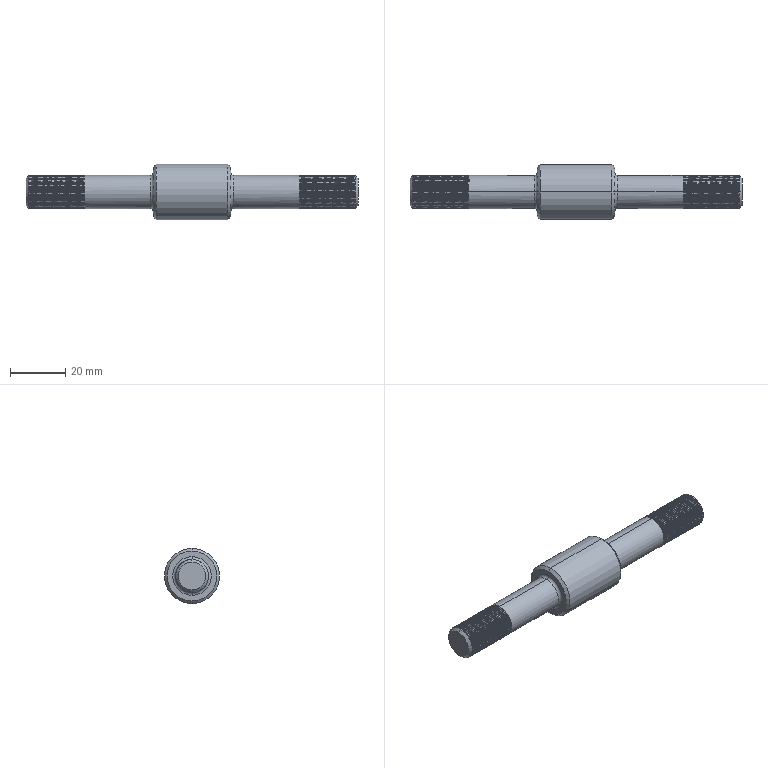Part | STEP file | Hinge pin stepped shaft 1 | 1 solid | 232 faces | box 120 x 20 x 20 mm | volume 18916 mm3 | cylinder 206 | cone 8 | plane 8 | spline 6 | torus 4 | commonest cylinder face diameters 12 x204 20 x2